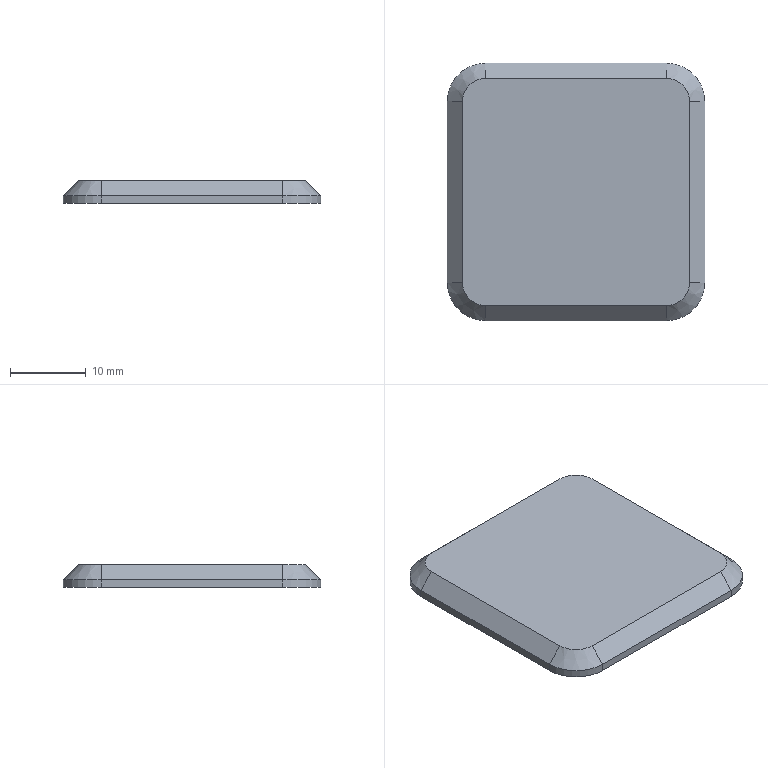Part | STEP file | IN-01-01-01-03 | 1 solid | 18 faces | box 34 x 34 x 3 mm | volume 3157 mm3 | plane 10 | cylinder 4 | cone 4 | commonest cylinder face diameters 10 x4
STEP:
#1=CARTESIAN_POINT('',(0.,0.,0.));
#2=DIRECTION('',(0.,0.,1.));
#3=DIRECTION('',(1.,0.,0.));
#4=AXIS2_PLACEMENT_3D('',#1,#2,#3);
#5=CARTESIAN_POINT('',(29.,-34.,0.));
#6=VERTEX_POINT('',#5);
#7=CARTESIAN_POINT('',(34.,-29.,0.));
#8=VERTEX_POINT('',#7);
#9=CARTESIAN_POINT('',(29.,-29.,0.));
#10=DIRECTION('',(0.,0.,1.));
#11=DIRECTION('',(1.,0.,0.));
#12=AXIS2_PLACEMENT_3D('',#9,#10,#11);
#13=CIRCLE('',#12,5.);
#14=CARTESIAN_POINT('',(17.,-17.,0.));
#15=DIRECTION('',(0.,0.,1.));
#16=DIRECTION('',(1.,0.,0.));
#17=AXIS2_PLACEMENT_3D('',#14,#15,#16);
#18=PLANE('',#17);
#19=CARTESIAN_POINT('',(12.,-12.));
#20=DIRECTION('',(1.,0.));
#21=AXIS2_PLACEMENT_2D('',#19,#20);
#22=CIRCLE('',#21,5.);
#23=(GEOMETRIC_REPRESENTATION_CONTEXT(2)PARAMETRIC_REPRESENTATION_CONTEXT()REPRESENTATION_CONTEXT('',''));
#24=DEFINITIONAL_REPRESENTATION('',(#22),#23);
#25=PCURVE('',#18,#24);
#26=CARTESIAN_POINT('',(29.,-29.,0.));
#27=DIRECTION('',(0.,0.,1.));
#28=DIRECTION('',(1.,0.,0.));
#29=AXIS2_PLACEMENT_3D('',#26,#27,#28);
#30=CYLINDRICAL_SURFACE('',#29,5.);
#31=CARTESIAN_POINT('',(0.,0.));
#32=DIRECTION('',(1.,0.));
#33=VECTOR('',#32,1.);
#34=LINE('',#31,#33);
#35=(GEOMETRIC_REPRESENTATION_CONTEXT(2)PARAMETRIC_REPRESENTATION_CONTEXT()REPRESENTATION_CONTEXT('',''));
#36=DEFINITIONAL_REPRESENTATION('',(#34),#35);
#37=PCURVE('',#30,#36);
#38=SURFACE_CURVE('',#13,(#25,#37),.PCURVE_S1.);
#39=EDGE_CURVE('',#6,#8,#38,.T.);
#40=ORIENTED_EDGE('',*,*,#39,.F.);
#41=CARTESIAN_POINT('',(5.,-34.,0.));
#42=VERTEX_POINT('',#41);
#43=CARTESIAN_POINT('',(17.,-34.,0.));
#44=DIRECTION('',(1.,0.,0.));
#45=VECTOR('',#44,1.);
#46=LINE('',#43,#45);
#47=CARTESIAN_POINT('',(0.,-17.));
#48=DIRECTION('',(1.,0.));
#49=VECTOR('',#48,1.);
#50=LINE('',#47,#49);
#51=(GEOMETRIC_REPRESENTATION_CONTEXT(2)PARAMETRIC_REPRESENTATION_CONTEXT()REPRESENTATION_CONTEXT('',''));
#52=DEFINITIONAL_REPRESENTATION('',(#50),#51);
#53=PCURVE('',#18,#52);
#54=CARTESIAN_POINT('',(5.,-34.,0.));
#55=DIRECTION('',(0.,-1.,0.));
#56=DIRECTION('',(1.,0.,0.));
#57=AXIS2_PLACEMENT_3D('',#54,#55,#56);
#58=PLANE('',#57);
#59=CARTESIAN_POINT('',(12.,0.));
#60=DIRECTION('',(1.,0.));
#61=VECTOR('',#60,1.);
#62=LINE('',#59,#61);
#63=(GEOMETRIC_REPRESENTATION_CONTEXT(2)PARAMETRIC_REPRESENTATION_CONTEXT()REPRESENTATION_CONTEXT('',''));
#64=DEFINITIONAL_REPRESENTATION('',(#62),#63);
#65=PCURVE('',#58,#64);
#66=SURFACE_CURVE('',#46,(#53,#65),.PCURVE_S1.);
#67=EDGE_CURVE('',#42,#6,#66,.T.);
#68=ORIENTED_EDGE('',*,*,#67,.F.);
#69=CARTESIAN_POINT('',(0.,-29.,0.));
#70=VERTEX_POINT('',#69);
#71=CARTESIAN_POINT('',(5.,-29.,0.));
#72=DIRECTION('',(0.,0.,1.));
#73=DIRECTION('',(1.,0.,0.));
#74=AXIS2_PLACEMENT_3D('',#71,#72,#73);
#75=CIRCLE('',#74,5.);
#76=CARTESIAN_POINT('',(-12.,-12.));
#77=DIRECTION('',(1.,0.));
#78=AXIS2_PLACEMENT_2D('',#76,#77);
#79=CIRCLE('',#78,5.);
#80=(GEOMETRIC_REPRESENTATION_CONTEXT(2)PARAMETRIC_REPRESENTATION_CONTEXT()REPRESENTATION_CONTEXT('',''));
#81=DEFINITIONAL_REPRESENTATION('',(#79),#80);
#82=PCURVE('',#18,#81);
#83=CARTESIAN_POINT('',(5.,-29.,0.));
#84=DIRECTION('',(0.,0.,1.));
#85=DIRECTION('',(1.,0.,0.));
#86=AXIS2_PLACEMENT_3D('',#83,#84,#85);
#87=CYLINDRICAL_SURFACE('',#86,5.);
#88=CARTESIAN_POINT('',(0.,0.));
#89=DIRECTION('',(1.,0.));
#90=VECTOR('',#89,1.);
#91=LINE('',#88,#90);
#92=(GEOMETRIC_REPRESENTATION_CONTEXT(2)PARAMETRIC_REPRESENTATION_CONTEXT()REPRESENTATION_CONTEXT('',''));
#93=DEFINITIONAL_REPRESENTATION('',(#91),#92);
#94=PCURVE('',#87,#93);
#95=SURFACE_CURVE('',#75,(#82,#94),.PCURVE_S1.);
#96=EDGE_CURVE('',#70,#42,#95,.T.);
#97=ORIENTED_EDGE('',*,*,#96,.F.);
#98=CARTESIAN_POINT('',(0.,-5.,0.));
#99=VERTEX_POINT('',#98);
#100=CARTESIAN_POINT('',(0.,-17.,0.));
#101=DIRECTION('',(0.,-1.,0.));
#102=VECTOR('',#101,1.);
#103=LINE('',#100,#102);
#104=CARTESIAN_POINT('',(-17.,0.));
#105=DIRECTION('',(0.,-1.));
#106=VECTOR('',#105,1.);
#107=LINE('',#104,#106);
#108=(GEOMETRIC_REPRESENTATION_CONTEXT(2)PARAMETRIC_REPRESENTATION_CONTEXT()REPRESENTATION_CONTEXT('',''));
#109=DEFINITIONAL_REPRESENTATION('',(#107),#108);
#110=PCURVE('',#18,#109);
#111=CARTESIAN_POINT('',(0.,-5.,0.));
#112=DIRECTION('',(-1.,0.,0.));
#113=DIRECTION('',(0.,-1.,0.));
#114=AXIS2_PLACEMENT_3D('',#111,#112,#113);
#115=PLANE('',#114);
#116=CARTESIAN_POINT('',(12.,0.));
#117=DIRECTION('',(1.,0.));
#118=VECTOR('',#117,1.);
#119=LINE('',#116,#118);
#120=(GEOMETRIC_REPRESENTATION_CONTEXT(2)PARAMETRIC_REPRESENTATION_CONTEXT()REPRESENTATION_CONTEXT('',''));
#121=DEFINITIONAL_REPRESENTATION('',(#119),#120);
#122=PCURVE('',#115,#121);
#123=SURFACE_CURVE('',#103,(#110,#122),.PCURVE_S1.);
#124=EDGE_CURVE('',#99,#70,#123,.T.);
#125=ORIENTED_EDGE('',*,*,#124,.F.);
#126=CARTESIAN_POINT('',(5.,0.,0.));
#127=VERTEX_POINT('',#126);
#128=CARTESIAN_POINT('',(5.,-5.,0.));
#129=DIRECTION('',(0.,0.,1.));
#130=DIRECTION('',(1.,0.,0.));
#131=AXIS2_PLACEMENT_3D('',#128,#129,#130);
#132=CIRCLE('',#131,5.);
#133=CARTESIAN_POINT('',(-12.,12.));
#134=DIRECTION('',(1.,0.));
#135=AXIS2_PLACEMENT_2D('',#133,#134);
#136=CIRCLE('',#135,5.);
#137=(GEOMETRIC_REPRESENTATION_CONTEXT(2)PARAMETRIC_REPRESENTATION_CONTEXT()REPRESENTATION_CONTEXT('',''));
#138=DEFINITIONAL_REPRESENTATION('',(#136),#137);
#139=PCURVE('',#18,#138);
#140=CARTESIAN_POINT('',(5.,-5.,0.));
#141=DIRECTION('',(0.,0.,1.));
#142=DIRECTION('',(1.,0.,0.));
#143=AXIS2_PLACEMENT_3D('',#140,#141,#142);
#144=CYLINDRICAL_SURFACE('',#143,5.);
#145=CARTESIAN_POINT('',(0.,0.));
#146=DIRECTION('',(1.,0.));
#147=VECTOR('',#146,1.);
#148=LINE('',#145,#147);
#149=(GEOMETRIC_REPRESENTATION_CONTEXT(2)PARAMETRIC_REPRESENTATION_CONTEXT()REPRESENTATION_CONTEXT('',''));
#150=DEFINITIONAL_REPRESENTATION('',(#148),#149);
#151=PCURVE('',#144,#150);
#152=SURFACE_CURVE('',#132,(#139,#151),.PCURVE_S1.);
#153=EDGE_CURVE('',#127,#99,#152,.T.);
#154=ORIENTED_EDGE('',*,*,#153,.F.);
#155=CARTESIAN_POINT('',(29.,0.,0.));
#156=VERTEX_POINT('',#155);
#157=CARTESIAN_POINT('',(17.,0.,0.));
#158=DIRECTION('',(-1.,0.,0.));
#159=VECTOR('',#158,1.);
#160=LINE('',#157,#159);
#161=CARTESIAN_POINT('',(0.,17.));
#162=DIRECTION('',(-1.,0.));
#163=VECTOR('',#162,1.);
#164=LINE('',#161,#163);
#165=(GEOMETRIC_REPRESENTATION_CONTEXT(2)PARAMETRIC_REPRESENTATION_CONTEXT()REPRESENTATION_CONTEXT('',''));
#166=DEFINITIONAL_REPRESENTATION('',(#164),#165);
#167=PCURVE('',#18,#166);
#168=CARTESIAN_POINT('',(29.,0.,0.));
#169=DIRECTION('',(0.,1.,0.));
#170=DIRECTION('',(-1.,0.,0.));
#171=AXIS2_PLACEMENT_3D('',#168,#169,#170);
#172=PLANE('',#171);
#173=CARTESIAN_POINT('',(12.,0.));
#174=DIRECTION('',(1.,0.));
#175=VECTOR('',#174,1.);
#176=LINE('',#173,#175);
#177=(GEOMETRIC_REPRESENTATION_CONTEXT(2)PARAMETRIC_REPRESENTATION_CONTEXT()REPRESENTATION_CONTEXT('',''));
#178=DEFINITIONAL_REPRESENTATION('',(#176),#177);
#179=PCURVE('',#172,#178);
#180=SURFACE_CURVE('',#160,(#167,#179),.PCURVE_S1.);
#181=EDGE_CURVE('',#156,#127,#180,.T.);
#182=ORIENTED_EDGE('',*,*,#181,.F.);
#183=CARTESIAN_POINT('',(34.,-5.,0.));
#184=VERTEX_POINT('',#183);
#185=CARTESIAN_POINT('',(29.,-5.,0.));
#186=DIRECTION('',(0.,0.,1.));
#187=DIRECTION('',(1.,0.,0.));
#188=AXIS2_PLACEMENT_3D('',#185,#186,#187);
#189=CIRCLE('',#188,5.);
#190=CARTESIAN_POINT('',(12.,12.));
#191=DIRECTION('',(1.,0.));
#192=AXIS2_PLACEMENT_2D('',#190,#191);
#193=CIRCLE('',#192,5.);
#194=(GEOMETRIC_REPRESENTATION_CONTEXT(2)PARAMETRIC_REPRESENTATION_CONTEXT()REPRESENTATION_CONTEXT('',''));
#195=DEFINITIONAL_REPRESENTATION('',(#193),#194);
#196=PCURVE('',#18,#195);
#197=CARTESIAN_POINT('',(29.,-5.,0.));
#198=DIRECTION('',(0.,0.,1.));
#199=DIRECTION('',(1.,0.,0.));
#200=AXIS2_PLACEMENT_3D('',#197,#198,#199);
#201=CYLINDRICAL_SURFACE('',#200,5.);
#202=CARTESIAN_POINT('',(0.,0.));
#203=DIRECTION('',(1.,0.));
#204=VECTOR('',#203,1.);
#205=LINE('',#202,#204);
#206=(GEOMETRIC_REPRESENTATION_CONTEXT(2)PARAMETRIC_REPRESENTATION_CONTEXT()REPRESENTATION_CONTEXT('',''));
#207=DEFINITIONAL_REPRESENTATION('',(#205),#206);
#208=PCURVE('',#201,#207);
#209=SURFACE_CURVE('',#189,(#196,#208),.PCURVE_S1.);
#210=EDGE_CURVE('',#184,#156,#209,.T.);
#211=ORIENTED_EDGE('',*,*,#210,.F.);
#212=CARTESIAN_POINT('',(34.,-17.,0.));
#213=DIRECTION('',(0.,1.,0.));
#214=VECTOR('',#213,1.);
#215=LINE('',#212,#214);
#216=CARTESIAN_POINT('',(17.,0.));
#217=DIRECTION('',(0.,1.));
#218=VECTOR('',#217,1.);
#219=LINE('',#216,#218);
#220=(GEOMETRIC_REPRESENTATION_CONTEXT(2)PARAMETRIC_REPRESENTATION_CONTEXT()REPRESENTATION_CONTEXT('',''));
#221=DEFINITIONAL_REPRESENTATION('',(#219),#220);
#222=PCURVE('',#18,#221);
#223=CARTESIAN_POINT('',(34.,-29.,0.));
#224=DIRECTION('',(1.,0.,0.));
#225=DIRECTION('',(0.,0.,-1.));
#226=AXIS2_PLACEMENT_3D('',#223,#224,#225);
#227=PLANE('',#226);
#228=CARTESIAN_POINT('',(0.,12.));
#229=DIRECTION('',(0.,1.));
#230=VECTOR('',#229,1.);
#231=LINE('',#228,#230);
#232=(GEOMETRIC_REPRESENTATION_CONTEXT(2)PARAMETRIC_REPRESENTATION_CONTEXT()REPRESENTATION_CONTEXT('',''));
#233=DEFINITIONAL_REPRESENTATION('',(#231),#232);
#234=PCURVE('',#227,#233);
#235=SURFACE_CURVE('',#215,(#222,#234),.PCURVE_S1.);
#236=EDGE_CURVE('',#8,#184,#235,.T.);
#237=ORIENTED_EDGE('',*,*,#236,.F.);
#238=EDGE_LOOP('',(#40,#68,#97,#125,#154,#182,#211,#237));
#239=FACE_BOUND('',#238,.T.);
#240=ADVANCED_FACE('',(#239),#18,.F.);
#241=ORIENTED_EDGE('',*,*,#236,.T.);
#242=CARTESIAN_POINT('',(34.,-5.,1.));
#243=VERTEX_POINT('',#242);
#244=CARTESIAN_POINT('',(34.,-5.,0.));
#245=DIRECTION('',(0.,0.,1.));
#246=VECTOR('',#245,1.);
#247=LINE('',#244,#246);
#248=CARTESIAN_POINT('',(0.,24.));
#249=DIRECTION('',(-1.,0.));
#250=VECTOR('',#249,1.);
#251=LINE('',#248,#250);
#252=(GEOMETRIC_REPRESENTATION_CONTEXT(2)PARAMETRIC_REPRESENTATION_CONTEXT()REPRESENTATION_CONTEXT('',''));
#253=DEFINITIONAL_REPRESENTATION('',(#251),#252);
#254=PCURVE('',#227,#253);
#255=CARTESIAN_POINT('',(0.,0.));
#256=DIRECTION('',(0.,1.));
#257=VECTOR('',#256,1.);
#258=LINE('',#255,#257);
#259=(GEOMETRIC_REPRESENTATION_CONTEXT(2)PARAMETRIC_REPRESENTATION_CONTEXT()REPRESENTATION_CONTEXT('',''));
#260=DEFINITIONAL_REPRESENTATION('',(#258),#259);
#261=PCURVE('',#201,#260);
#262=SURFACE_CURVE('',#247,(#254,#261),.PCURVE_S1.);
#263=EDGE_CURVE('',#184,#243,#262,.T.);
#264=ORIENTED_EDGE('',*,*,#263,.T.);
#265=CARTESIAN_POINT('',(34.,-29.,1.));
#266=VERTEX_POINT('',#265);
#267=CARTESIAN_POINT('',(34.,-29.,1.));
#268=DIRECTION('',(0.,-1.,0.));
#269=VECTOR('',#268,1.);
#270=LINE('',#267,#269);
#271=CARTESIAN_POINT('',(-1.,0.));
#272=DIRECTION('',(0.,-1.));
#273=VECTOR('',#272,1.);
#274=LINE('',#271,#273);
#275=(GEOMETRIC_REPRESENTATION_CONTEXT(2)PARAMETRIC_REPRESENTATION_CONTEXT()REPRESENTATION_CONTEXT('',''));
#276=DEFINITIONAL_REPRESENTATION('',(#274),#275);
#277=PCURVE('',#227,#276);
#278=CARTESIAN_POINT('',(33.,-23.,2.));
#279=DIRECTION('',(0.7071,0.,0.7071));
#280=DIRECTION('',(0.7071,0.,-0.7071));
#281=AXIS2_PLACEMENT_3D('',#278,#279,#280);
#282=PLANE('',#281);
#283=CARTESIAN_POINT('',(1.414,-6.));
#284=DIRECTION('',(0.,-1.));
#285=VECTOR('',#284,1.);
#286=LINE('',#283,#285);
#287=(GEOMETRIC_REPRESENTATION_CONTEXT(2)PARAMETRIC_REPRESENTATION_CONTEXT()REPRESENTATION_CONTEXT('',''));
#288=DEFINITIONAL_REPRESENTATION('',(#286),#287);
#289=PCURVE('',#282,#288);
#290=SURFACE_CURVE('',#270,(#277,#289),.PCURVE_S1.);
#291=EDGE_CURVE('',#243,#266,#290,.T.);
#292=ORIENTED_EDGE('',*,*,#291,.T.);
#293=CARTESIAN_POINT('',(34.,-29.,0.));
#294=DIRECTION('',(0.,0.,-1.));
#295=VECTOR('',#294,1.);
#296=LINE('',#293,#295);
#297=CARTESIAN_POINT('',(0.,0.));
#298=DIRECTION('',(1.,0.));
#299=VECTOR('',#298,1.);
#300=LINE('',#297,#299);
#301=(GEOMETRIC_REPRESENTATION_CONTEXT(2)PARAMETRIC_REPRESENTATION_CONTEXT()REPRESENTATION_CONTEXT('',''));
#302=DEFINITIONAL_REPRESENTATION('',(#300),#301);
#303=PCURVE('',#227,#302);
#304=CARTESIAN_POINT('',(6.283,0.));
#305=DIRECTION('',(0.,-1.));
#306=VECTOR('',#305,1.);
#307=LINE('',#304,#306);
#308=(GEOMETRIC_REPRESENTATION_CONTEXT(2)PARAMETRIC_REPRESENTATION_CONTEXT()REPRESENTATION_CONTEXT('',''));
#309=DEFINITIONAL_REPRESENTATION('',(#307),#308);
#310=PCURVE('',#30,#309);
#311=SURFACE_CURVE('',#296,(#303,#310),.PCURVE_S1.);
#312=EDGE_CURVE('',#266,#8,#311,.T.);
#313=ORIENTED_EDGE('',*,*,#312,.T.);
#314=EDGE_LOOP('',(#241,#264,#292,#313));
#315=FACE_BOUND('',#314,.T.);
#316=ADVANCED_FACE('',(#315),#227,.T.);
#317=ORIENTED_EDGE('',*,*,#39,.T.);
#318=ORIENTED_EDGE('',*,*,#312,.F.);
#319=CARTESIAN_POINT('',(29.,-34.,1.));
#320=VERTEX_POINT('',#319);
#321=CARTESIAN_POINT('',(29.,-29.,1.));
#322=DIRECTION('',(0.,0.,-1.));
#323=DIRECTION('',(1.,0.,0.));
#324=AXIS2_PLACEMENT_3D('',#321,#322,#323);
#325=CIRCLE('',#324,5.);
#326=CARTESIAN_POINT('',(6.283,1.));
#327=DIRECTION('',(-1.,0.));
#328=VECTOR('',#327,1.);
#329=LINE('',#326,#328);
#330=(GEOMETRIC_REPRESENTATION_CONTEXT(2)PARAMETRIC_REPRESENTATION_CONTEXT()REPRESENTATION_CONTEXT('',''));
#331=DEFINITIONAL_REPRESENTATION('',(#329),#330);
#332=PCURVE('',#30,#331);
#333=CARTESIAN_POINT('',(29.,-29.,1.));
#334=DIRECTION('',(0.,0.,-1.));
#335=DIRECTION('',(-1.,0.,0.));
#336=AXIS2_PLACEMENT_3D('',#333,#334,#335);
#337=CONICAL_SURFACE('',#336,5.,0.7854);
#338=CARTESIAN_POINT('',(3.142,0.));
#339=DIRECTION('',(1.,0.));
#340=VECTOR('',#339,1.);
#341=LINE('',#338,#340);
#342=(GEOMETRIC_REPRESENTATION_CONTEXT(2)PARAMETRIC_REPRESENTATION_CONTEXT()REPRESENTATION_CONTEXT('',''));
#343=DEFINITIONAL_REPRESENTATION('',(#341),#342);
#344=PCURVE('',#337,#343);
#345=SURFACE_CURVE('',#325,(#332,#344),.PCURVE_S1.);
#346=EDGE_CURVE('',#266,#320,#345,.T.);
#347=ORIENTED_EDGE('',*,*,#346,.T.);
#348=CARTESIAN_POINT('',(29.,-34.,0.));
#349=DIRECTION('',(0.,0.,-1.));
#350=VECTOR('',#349,1.);
#351=LINE('',#348,#350);
#352=CARTESIAN_POINT('',(4.712,0.));
#353=DIRECTION('',(0.,-1.));
#354=VECTOR('',#353,1.);
#355=LINE('',#352,#354);
#356=(GEOMETRIC_REPRESENTATION_CONTEXT(2)PARAMETRIC_REPRESENTATION_CONTEXT()REPRESENTATION_CONTEXT('',''));
#357=DEFINITIONAL_REPRESENTATION('',(#355),#356);
#358=PCURVE('',#30,#357);
#359=CARTESIAN_POINT('',(24.,0.));
#360=DIRECTION('',(0.,-1.));
#361=VECTOR('',#360,1.);
#362=LINE('',#359,#361);
#363=(GEOMETRIC_REPRESENTATION_CONTEXT(2)PARAMETRIC_REPRESENTATION_CONTEXT()REPRESENTATION_CONTEXT('',''));
#364=DEFINITIONAL_REPRESENTATION('',(#362),#363);
#365=PCURVE('',#58,#364);
#366=SURFACE_CURVE('',#351,(#358,#365),.PCURVE_S1.);
#367=EDGE_CURVE('',#320,#6,#366,.T.);
#368=ORIENTED_EDGE('',*,*,#367,.T.);
#369=EDGE_LOOP('',(#317,#318,#347,#368));
#370=FACE_BOUND('',#369,.T.);
#371=ADVANCED_FACE('',(#370),#30,.T.);
#372=ORIENTED_EDGE('',*,*,#67,.T.);
#373=ORIENTED_EDGE('',*,*,#367,.F.);
#374=CARTESIAN_POINT('',(5.,-34.,1.));
#375=VERTEX_POINT('',#374);
#376=CARTESIAN_POINT('',(5.,-34.,1.));
#377=DIRECTION('',(-1.,0.,0.));
#378=VECTOR('',#377,1.);
#379=LINE('',#376,#378);
#380=CARTESIAN_POINT('',(0.,1.));
#381=DIRECTION('',(-1.,0.));
#382=VECTOR('',#381,1.);
#383=LINE('',#380,#382);
#384=(GEOMETRIC_REPRESENTATION_CONTEXT(2)PARAMETRIC_REPRESENTATION_CONTEXT()REPRESENTATION_CONTEXT('',''));
#385=DEFINITIONAL_REPRESENTATION('',(#383),#384);
#386=PCURVE('',#58,#385);
#387=CARTESIAN_POINT('',(11.,-33.,2.));
#388=DIRECTION('',(0.,-0.7071,0.7071));
#389=DIRECTION('',(0.,-0.7071,-0.7071));
#390=AXIS2_PLACEMENT_3D('',#387,#388,#389);
#391=PLANE('',#390);
#392=CARTESIAN_POINT('',(1.414,-6.));
#393=DIRECTION('',(0.,-1.));
#394=VECTOR('',#393,1.);
#395=LINE('',#392,#394);
#396=(GEOMETRIC_REPRESENTATION_CONTEXT(2)PARAMETRIC_REPRESENTATION_CONTEXT()REPRESENTATION_CONTEXT('',''));
#397=DEFINITIONAL_REPRESENTATION('',(#395),#396);
#398=PCURVE('',#391,#397);
#399=SURFACE_CURVE('',#379,(#386,#398),.PCURVE_S1.);
#400=EDGE_CURVE('',#320,#375,#399,.T.);
#401=ORIENTED_EDGE('',*,*,#400,.T.);
#402=CARTESIAN_POINT('',(5.,-34.,0.));
#403=DIRECTION('',(0.,0.,-1.));
#404=VECTOR('',#403,1.);
#405=LINE('',#402,#404);
#406=CARTESIAN_POINT('',(0.,0.));
#407=DIRECTION('',(0.,-1.));
#408=VECTOR('',#407,1.);
#409=LINE('',#406,#408);
#410=(GEOMETRIC_REPRESENTATION_CONTEXT(2)PARAMETRIC_REPRESENTATION_CONTEXT()REPRESENTATION_CONTEXT('',''));
#411=DEFINITIONAL_REPRESENTATION('',(#409),#410);
#412=PCURVE('',#58,#411);
#413=CARTESIAN_POINT('',(4.712,0.));
#414=DIRECTION('',(0.,-1.));
#415=VECTOR('',#414,1.);
#416=LINE('',#413,#415);
#417=(GEOMETRIC_REPRESENTATION_CONTEXT(2)PARAMETRIC_REPRESENTATION_CONTEXT()REPRESENTATION_CONTEXT('',''));
#418=DEFINITIONAL_REPRESENTATION('',(#416),#417);
#419=PCURVE('',#87,#418);
#420=SURFACE_CURVE('',#405,(#412,#419),.PCURVE_S1.);
#421=EDGE_CURVE('',#375,#42,#420,.T.);
#422=ORIENTED_EDGE('',*,*,#421,.T.);
#423=EDGE_LOOP('',(#372,#373,#401,#422));
#424=FACE_BOUND('',#423,.T.);
#425=ADVANCED_FACE('',(#424),#58,.T.);
#426=ORIENTED_EDGE('',*,*,#96,.T.);
#427=ORIENTED_EDGE('',*,*,#421,.F.);
#428=CARTESIAN_POINT('',(0.,-29.,1.));
#429=VERTEX_POINT('',#428);
#430=CARTESIAN_POINT('',(5.,-29.,1.));
#431=DIRECTION('',(0.,0.,-1.));
#432=DIRECTION('',(1.,0.,0.));
#433=AXIS2_PLACEMENT_3D('',#430,#431,#432);
#434=CIRCLE('',#433,5.);
#435=CARTESIAN_POINT('',(6.283,1.));
#436=DIRECTION('',(-1.,0.));
#437=VECTOR('',#436,1.);
#438=LINE('',#435,#437);
#439=(GEOMETRIC_REPRESENTATION_CONTEXT(2)PARAMETRIC_REPRESENTATION_CONTEXT()REPRESENTATION_CONTEXT('',''));
#440=DEFINITIONAL_REPRESENTATION('',(#438),#439);
#441=PCURVE('',#87,#440);
#442=CARTESIAN_POINT('',(5.,-29.,1.));
#443=DIRECTION('',(0.,0.,-1.));
#444=DIRECTION('',(-1.,0.,0.));
#445=AXIS2_PLACEMENT_3D('',#442,#443,#444);
#446=CONICAL_SURFACE('',#445,5.,0.7854);
#447=CARTESIAN_POINT('',(3.142,0.));
#448=DIRECTION('',(1.,0.));
#449=VECTOR('',#448,1.);
#450=LINE('',#447,#449);
#451=(GEOMETRIC_REPRESENTATION_CONTEXT(2)PARAMETRIC_REPRESENTATION_CONTEXT()REPRESENTATION_CONTEXT('',''));
#452=DEFINITIONAL_REPRESENTATION('',(#450),#451);
#453=PCURVE('',#446,#452);
#454=SURFACE_CURVE('',#434,(#441,#453),.PCURVE_S1.);
#455=EDGE_CURVE('',#375,#429,#454,.T.);
#456=ORIENTED_EDGE('',*,*,#455,.T.);
#457=CARTESIAN_POINT('',(0.,-29.,0.));
#458=DIRECTION('',(0.,0.,-1.));
#459=VECTOR('',#458,1.);
#460=LINE('',#457,#459);
#461=CARTESIAN_POINT('',(3.142,0.));
#462=DIRECTION('',(0.,-1.));
#463=VECTOR('',#462,1.);
#464=LINE('',#461,#463);
#465=(GEOMETRIC_REPRESENTATION_CONTEXT(2)PARAMETRIC_REPRESENTATION_CONTEXT()REPRESENTATION_CONTEXT('',''));
#466=DEFINITIONAL_REPRESENTATION('',(#464),#465);
#467=PCURVE('',#87,#466);
#468=CARTESIAN_POINT('',(24.,0.));
#469=DIRECTION('',(0.,-1.));
#470=VECTOR('',#469,1.);
#471=LINE('',#468,#470);
#472=(GEOMETRIC_REPRESENTATION_CONTEXT(2)PARAMETRIC_REPRESENTATION_CONTEXT()REPRESENTATION_CONTEXT('',''));
#473=DEFINITIONAL_REPRESENTATION('',(#471),#472);
#474=PCURVE('',#115,#473);
#475=SURFACE_CURVE('',#460,(#467,#474),.PCURVE_S1.);
#476=EDGE_CURVE('',#429,#70,#475,.T.);
#477=ORIENTED_EDGE('',*,*,#476,.T.);
#478=EDGE_LOOP('',(#426,#427,#456,#477));
#479=FACE_BOUND('',#478,.T.);
#480=ADVANCED_FACE('',(#479),#87,.T.);
#481=ORIENTED_EDGE('',*,*,#124,.T.);
#482=ORIENTED_EDGE('',*,*,#476,.F.);
#483=CARTESIAN_POINT('',(0.,-5.,1.));
#484=VERTEX_POINT('',#483);
#485=CARTESIAN_POINT('',(0.,-5.,1.));
#486=DIRECTION('',(0.,1.,0.));
#487=VECTOR('',#486,1.);
#488=LINE('',#485,#487);
#489=CARTESIAN_POINT('',(0.,1.));
#490=DIRECTION('',(-1.,0.));
#491=VECTOR('',#490,1.);
#492=LINE('',#489,#491);
#493=(GEOMETRIC_REPRESENTATION_CONTEXT(2)PARAMETRIC_REPRESENTATION_CONTEXT()REPRESENTATION_CONTEXT('',''));
#494=DEFINITIONAL_REPRESENTATION('',(#492),#493);
#495=PCURVE('',#115,#494);
#496=CARTESIAN_POINT('',(1.,-11.,2.));
#497=DIRECTION('',(-0.7071,0.,0.7071));
#498=DIRECTION('',(0.7071,0.,0.7071));
#499=AXIS2_PLACEMENT_3D('',#496,#497,#498);
#500=PLANE('',#499);
#501=CARTESIAN_POINT('',(-1.414,6.));
#502=DIRECTION('',(0.,1.));
#503=VECTOR('',#502,1.);
#504=LINE('',#501,#503);
#505=(GEOMETRIC_REPRESENTATION_CONTEXT(2)PARAMETRIC_REPRESENTATION_CONTEXT()REPRESENTATION_CONTEXT('',''));
#506=DEFINITIONAL_REPRESENTATION('',(#504),#505);
#507=PCURVE('',#500,#506);
#508=SURFACE_CURVE('',#488,(#495,#507),.PCURVE_S1.);
#509=EDGE_CURVE('',#429,#484,#508,.T.);
#510=ORIENTED_EDGE('',*,*,#509,.T.);
#511=CARTESIAN_POINT('',(0.,-5.,0.));
#512=DIRECTION('',(0.,0.,-1.));
#513=VECTOR('',#512,1.);
#514=LINE('',#511,#513);
#515=CARTESIAN_POINT('',(0.,0.));
#516=DIRECTION('',(0.,-1.));
#517=VECTOR('',#516,1.);
#518=LINE('',#515,#517);
#519=(GEOMETRIC_REPRESENTATION_CONTEXT(2)PARAMETRIC_REPRESENTATION_CONTEXT()REPRESENTATION_CONTEXT('',''));
#520=DEFINITIONAL_REPRESENTATION('',(#518),#519);
#521=PCURVE('',#115,#520);
#522=CARTESIAN_POINT('',(3.142,0.));
#523=DIRECTION('',(0.,-1.));
#524=VECTOR('',#523,1.);
#525=LINE('',#522,#524);
#526=(GEOMETRIC_REPRESENTATION_CONTEXT(2)PARAMETRIC_REPRESENTATION_CONTEXT()REPRESENTATION_CONTEXT('',''));
#527=DEFINITIONAL_REPRESENTATION('',(#525),#526);
#528=PCURVE('',#144,#527);
#529=SURFACE_CURVE('',#514,(#521,#528),.PCURVE_S1.);
#530=EDGE_CURVE('',#484,#99,#529,.T.);
#531=ORIENTED_EDGE('',*,*,#530,.T.);
#532=EDGE_LOOP('',(#481,#482,#510,#531));
#533=FACE_BOUND('',#532,.T.);
#534=ADVANCED_FACE('',(#533),#115,.T.);
#535=ORIENTED_EDGE('',*,*,#153,.T.);
#536=ORIENTED_EDGE('',*,*,#530,.F.);
#537=CARTESIAN_POINT('',(5.,0.,1.));
#538=VERTEX_POINT('',#537);
#539=CARTESIAN_POINT('',(5.,-5.,1.));
#540=DIRECTION('',(0.,0.,-1.));
#541=DIRECTION('',(1.,0.,0.));
#542=AXIS2_PLACEMENT_3D('',#539,#540,#541);
#543=CIRCLE('',#542,5.);
#544=CARTESIAN_POINT('',(6.283,1.));
#545=DIRECTION('',(-1.,0.));
#546=VECTOR('',#545,1.);
#547=LINE('',#544,#546);
#548=(GEOMETRIC_REPRESENTATION_CONTEXT(2)PARAMETRIC_REPRESENTATION_CONTEXT()REPRESENTATION_CONTEXT('',''));
#549=DEFINITIONAL_REPRESENTATION('',(#547),#548);
#550=PCURVE('',#144,#549);
#551=CARTESIAN_POINT('',(5.,-5.,1.));
#552=DIRECTION('',(0.,0.,-1.));
#553=DIRECTION('',(-1.,0.,0.));
#554=AXIS2_PLACEMENT_3D('',#551,#552,#553);
#555=CONICAL_SURFACE('',#554,5.,0.7854);
#556=CARTESIAN_POINT('',(-3.142,0.));
#557=DIRECTION('',(1.,0.));
#558=VECTOR('',#557,1.);
#559=LINE('',#556,#558);
#560=(GEOMETRIC_REPRESENTATION_CONTEXT(2)PARAMETRIC_REPRESENTATION_CONTEXT()REPRESENTATION_CONTEXT('',''));
#561=DEFINITIONAL_REPRESENTATION('',(#559),#560);
#562=PCURVE('',#555,#561);
#563=SURFACE_CURVE('',#543,(#550,#562),.PCURVE_S1.);
#564=EDGE_CURVE('',#484,#538,#563,.T.);
#565=ORIENTED_EDGE('',*,*,#564,.T.);
#566=CARTESIAN_POINT('',(5.,0.,0.));
#567=DIRECTION('',(0.,0.,-1.));
#568=VECTOR('',#567,1.);
#569=LINE('',#566,#568);
#570=CARTESIAN_POINT('',(1.571,0.));
#571=DIRECTION('',(0.,-1.));
#572=VECTOR('',#571,1.);
#573=LINE('',#570,#572);
#574=(GEOMETRIC_REPRESENTATION_CONTEXT(2)PARAMETRIC_REPRESENTATION_CONTEXT()REPRESENTATION_CONTEXT('',''));
#575=DEFINITIONAL_REPRESENTATION('',(#573),#574);
#576=PCURVE('',#144,#575);
#577=CARTESIAN_POINT('',(24.,0.));
#578=DIRECTION('',(0.,-1.));
#579=VECTOR('',#578,1.);
#580=LINE('',#577,#579);
#581=(GEOMETRIC_REPRESENTATION_CONTEXT(2)PARAMETRIC_REPRESENTATION_CONTEXT()REPRESENTATION_CONTEXT('',''));
#582=DEFINITIONAL_REPRESENTATION('',(#580),#581);
#583=PCURVE('',#172,#582);
#584=SURFACE_CURVE('',#569,(#576,#583),.PCURVE_S1.);
#585=EDGE_CURVE('',#538,#127,#584,.T.);
#586=ORIENTED_EDGE('',*,*,#585,.T.);
#587=EDGE_LOOP('',(#535,#536,#565,#586));
#588=FACE_BOUND('',#587,.T.);
#589=ADVANCED_FACE('',(#588),#144,.T.);
#590=ORIENTED_EDGE('',*,*,#181,.T.);
#591=ORIENTED_EDGE('',*,*,#585,.F.);
#592=CARTESIAN_POINT('',(29.,0.,1.));
#593=VERTEX_POINT('',#592);
#594=CARTESIAN_POINT('',(29.,0.,1.));
#595=DIRECTION('',(1.,0.,0.));
#596=VECTOR('',#595,1.);
#597=LINE('',#594,#596);
#598=CARTESIAN_POINT('',(0.,1.));
#599=DIRECTION('',(-1.,0.));
#600=VECTOR('',#599,1.);
#601=LINE('',#598,#600);
#602=(GEOMETRIC_REPRESENTATION_CONTEXT(2)PARAMETRIC_REPRESENTATION_CONTEXT()REPRESENTATION_CONTEXT('',''));
#603=DEFINITIONAL_REPRESENTATION('',(#601),#602);
#604=PCURVE('',#172,#603);
#605=CARTESIAN_POINT('',(23.,-1.,2.));
#606=DIRECTION('',(0.,0.7071,0.7071));
#607=DIRECTION('',(0.,-0.7071,0.7071));
#608=AXIS2_PLACEMENT_3D('',#605,#606,#607);
#609=PLANE('',#608);
#610=CARTESIAN_POINT('',(-1.414,6.));
#611=DIRECTION('',(0.,1.));
#612=VECTOR('',#611,1.);
#613=LINE('',#610,#612);
#614=(GEOMETRIC_REPRESENTATION_CONTEXT(2)PARAMETRIC_REPRESENTATION_CONTEXT()REPRESENTATION_CONTEXT('',''));
#615=DEFINITIONAL_REPRESENTATION('',(#613),#614);
#616=PCURVE('',#609,#615);
#617=SURFACE_CURVE('',#597,(#604,#616),.PCURVE_S1.);
#618=EDGE_CURVE('',#538,#593,#617,.T.);
#619=ORIENTED_EDGE('',*,*,#618,.T.);
#620=CARTESIAN_POINT('',(29.,0.,0.));
#621=DIRECTION('',(0.,0.,-1.));
#622=VECTOR('',#621,1.);
#623=LINE('',#620,#622);
#624=CARTESIAN_POINT('',(0.,0.));
#625=DIRECTION('',(0.,-1.));
#626=VECTOR('',#625,1.);
#627=LINE('',#624,#626);
#628=(GEOMETRIC_REPRESENTATION_CONTEXT(2)PARAMETRIC_REPRESENTATION_CONTEXT()REPRESENTATION_CONTEXT('',''));
#629=DEFINITIONAL_REPRESENTATION('',(#627),#628);
#630=PCURVE('',#172,#629);
#631=CARTESIAN_POINT('',(1.571,0.));
#632=DIRECTION('',(0.,-1.));
#633=VECTOR('',#632,1.);
#634=LINE('',#631,#633);
#635=(GEOMETRIC_REPRESENTATION_CONTEXT(2)PARAMETRIC_REPRESENTATION_CONTEXT()REPRESENTATION_CONTEXT('',''));
#636=DEFINITIONAL_REPRESENTATION('',(#634),#635);
#637=PCURVE('',#201,#636);
#638=SURFACE_CURVE('',#623,(#630,#637),.PCURVE_S1.);
#639=EDGE_CURVE('',#593,#156,#638,.T.);
#640=ORIENTED_EDGE('',*,*,#639,.T.);
#641=EDGE_LOOP('',(#590,#591,#619,#640));
#642=FACE_BOUND('',#641,.T.);
#643=ADVANCED_FACE('',(#642),#172,.T.);
#644=ORIENTED_EDGE('',*,*,#210,.T.);
#645=ORIENTED_EDGE('',*,*,#639,.F.);
#646=CARTESIAN_POINT('',(29.,-5.,1.));
#647=DIRECTION('',(0.,0.,-1.));
#648=DIRECTION('',(1.,0.,0.));
#649=AXIS2_PLACEMENT_3D('',#646,#647,#648);
#650=CIRCLE('',#649,5.);
#651=CARTESIAN_POINT('',(6.283,1.));
#652=DIRECTION('',(-1.,0.));
#653=VECTOR('',#652,1.);
#654=LINE('',#651,#653);
#655=(GEOMETRIC_REPRESENTATION_CONTEXT(2)PARAMETRIC_REPRESENTATION_CONTEXT()REPRESENTATION_CONTEXT('',''));
#656=DEFINITIONAL_REPRESENTATION('',(#654),#655);
#657=PCURVE('',#201,#656);
#658=CARTESIAN_POINT('',(29.,-5.,1.));
#659=DIRECTION('',(0.,0.,-1.));
#660=DIRECTION('',(-1.,0.,0.));
#661=AXIS2_PLACEMENT_3D('',#658,#659,#660);
#662=CONICAL_SURFACE('',#661,5.,0.7854);
#663=CARTESIAN_POINT('',(-3.142,0.));
#664=DIRECTION('',(1.,0.));
#665=VECTOR('',#664,1.);
#666=LINE('',#663,#665);
#667=(GEOMETRIC_REPRESENTATION_CONTEXT(2)PARAMETRIC_REPRESENTATION_CONTEXT()REPRESENTATION_CONTEXT('',''));
#668=DEFINITIONAL_REPRESENTATION('',(#666),#667);
#669=PCURVE('',#662,#668);
#670=SURFACE_CURVE('',#650,(#657,#669),.PCURVE_S1.);
#671=EDGE_CURVE('',#593,#243,#670,.T.);
#672=ORIENTED_EDGE('',*,*,#671,.T.);
#673=ORIENTED_EDGE('',*,*,#263,.F.);
#674=EDGE_LOOP('',(#644,#645,#672,#673));
#675=FACE_BOUND('',#674,.T.);
#676=ADVANCED_FACE('',(#675),#201,.T.);
#677=CARTESIAN_POINT('',(32.,-29.,3.));
#678=VERTEX_POINT('',#677);
#679=CARTESIAN_POINT('',(33.,-29.,2.));
#680=DIRECTION('',(0.7071,0.,-0.7071));
#681=VECTOR('',#680,1.);
#682=LINE('',#679,#681);
#683=CARTESIAN_POINT('',(0.,-6.));
#684=DIRECTION('',(1.,0.));
#685=VECTOR('',#684,1.);
#686=LINE('',#683,#685);
#687=(GEOMETRIC_REPRESENTATION_CONTEXT(2)PARAMETRIC_REPRESENTATION_CONTEXT()REPRESENTATION_CONTEXT('',''));
#688=DEFINITIONAL_REPRESENTATION('',(#686),#687);
#689=PCURVE('',#282,#688);
#690=CARTESIAN_POINT('',(3.142,-1.));
#691=DIRECTION('',(0.,1.));
#692=VECTOR('',#691,1.);
#693=LINE('',#690,#692);
#694=(GEOMETRIC_REPRESENTATION_CONTEXT(2)PARAMETRIC_REPRESENTATION_CONTEXT()REPRESENTATION_CONTEXT('',''));
#695=DEFINITIONAL_REPRESENTATION('',(#693),#694);
#696=PCURVE('',#337,#695);
#697=SURFACE_CURVE('',#682,(#689,#696),.PCURVE_S1.);
#698=EDGE_CURVE('',#678,#266,#697,.T.);
#699=ORIENTED_EDGE('',*,*,#698,.T.);
#700=ORIENTED_EDGE('',*,*,#291,.F.);
#701=CARTESIAN_POINT('',(32.,-5.,3.));
#702=VERTEX_POINT('',#701);
#703=CARTESIAN_POINT('',(33.,-5.,2.));
#704=DIRECTION('',(-0.7071,0.,0.7071));
#705=VECTOR('',#704,1.);
#706=LINE('',#703,#705);
#707=CARTESIAN_POINT('',(0.,18.));
#708=DIRECTION('',(-1.,0.));
#709=VECTOR('',#708,1.);
#710=LINE('',#707,#709);
#711=(GEOMETRIC_REPRESENTATION_CONTEXT(2)PARAMETRIC_REPRESENTATION_CONTEXT()REPRESENTATION_CONTEXT('',''));
#712=DEFINITIONAL_REPRESENTATION('',(#710),#711);
#713=PCURVE('',#282,#712);
#714=CARTESIAN_POINT('',(3.142,-1.));
#715=DIRECTION('',(0.,-1.));
#716=VECTOR('',#715,1.);
#717=LINE('',#714,#716);
#718=(GEOMETRIC_REPRESENTATION_CONTEXT(2)PARAMETRIC_REPRESENTATION_CONTEXT()REPRESENTATION_CONTEXT('',''));
#719=DEFINITIONAL_REPRESENTATION('',(#717),#718);
#720=PCURVE('',#662,#719);
#721=SURFACE_CURVE('',#706,(#713,#720),.PCURVE_S1.);
#722=EDGE_CURVE('',#243,#702,#721,.T.);
#723=ORIENTED_EDGE('',*,*,#722,.T.);
#724=CARTESIAN_POINT('',(32.,-23.,3.));
#725=DIRECTION('',(0.,-1.,0.));
#726=VECTOR('',#725,1.);
#727=LINE('',#724,#726);
#728=CARTESIAN_POINT('',(-1.414,0.));
#729=DIRECTION('',(0.,-1.));
#730=VECTOR('',#729,1.);
#731=LINE('',#728,#730);
#732=(GEOMETRIC_REPRESENTATION_CONTEXT(2)PARAMETRIC_REPRESENTATION_CONTEXT()REPRESENTATION_CONTEXT('',''));
#733=DEFINITIONAL_REPRESENTATION('',(#731),#732);
#734=PCURVE('',#282,#733);
#735=CARTESIAN_POINT('',(17.,-17.,3.));
#736=DIRECTION('',(0.,0.,1.));
#737=DIRECTION('',(1.,0.,0.));
#738=AXIS2_PLACEMENT_3D('',#735,#736,#737);
#739=PLANE('',#738);
#740=CARTESIAN_POINT('',(15.,-6.));
#741=DIRECTION('',(0.,-1.));
#742=VECTOR('',#741,1.);
#743=LINE('',#740,#742);
#744=(GEOMETRIC_REPRESENTATION_CONTEXT(2)PARAMETRIC_REPRESENTATION_CONTEXT()REPRESENTATION_CONTEXT('',''));
#745=DEFINITIONAL_REPRESENTATION('',(#743),#744);
#746=PCURVE('',#739,#745);
#747=SURFACE_CURVE('',#727,(#734,#746),.PCURVE_S1.);
#748=EDGE_CURVE('',#702,#678,#747,.T.);
#749=ORIENTED_EDGE('',*,*,#748,.T.);
#750=EDGE_LOOP('',(#699,#700,#723,#749));
#751=FACE_BOUND('',#750,.T.);
#752=ADVANCED_FACE('',(#751),#282,.T.);
#753=CARTESIAN_POINT('',(29.,-32.,3.));
#754=VERTEX_POINT('',#753);
#755=CARTESIAN_POINT('',(29.,-499000.,-498965.));
#756=DIRECTION('',(0.,-0.7071,-0.7071));
#757=VECTOR('',#756,1.);
#758=LINE('',#755,#757);
#759=CARTESIAN_POINT('',(4.712,498966.));
#760=DIRECTION('',(0.,1.));
#761=VECTOR('',#760,1.);
#762=LINE('',#759,#761);
#763=(GEOMETRIC_REPRESENTATION_CONTEXT(2)PARAMETRIC_REPRESENTATION_CONTEXT()REPRESENTATION_CONTEXT('',''));
#764=DEFINITIONAL_REPRESENTATION('',(#762),#763);
#765=PCURVE('',#337,#764);
#766=CARTESIAN_POINT('',(705645.899,18.));
#767=DIRECTION('',(1.,0.));
#768=VECTOR('',#767,1.);
#769=LINE('',#766,#768);
#770=(GEOMETRIC_REPRESENTATION_CONTEXT(2)PARAMETRIC_REPRESENTATION_CONTEXT()REPRESENTATION_CONTEXT('',''));
#771=DEFINITIONAL_REPRESENTATION('',(#769),#770);
#772=PCURVE('',#391,#771);
#773=SURFACE_CURVE('',#758,(#765,#772),.PCURVE_S1.);
#774=EDGE_CURVE('',#754,#320,#773,.T.);
#775=ORIENTED_EDGE('',*,*,#774,.T.);
#776=ORIENTED_EDGE('',*,*,#346,.F.);
#777=ORIENTED_EDGE('',*,*,#698,.F.);
#778=CARTESIAN_POINT('',(29.,-29.,3.));
#779=DIRECTION('',(0.,0.,-1.));
#780=DIRECTION('',(-1.,0.,0.));
#781=AXIS2_PLACEMENT_3D('',#778,#779,#780);
#782=CIRCLE('',#781,3.);
#783=CARTESIAN_POINT('',(0.,-2.));
#784=DIRECTION('',(1.,0.));
#785=VECTOR('',#784,1.);
#786=LINE('',#783,#785);
#787=(GEOMETRIC_REPRESENTATION_CONTEXT(2)PARAMETRIC_REPRESENTATION_CONTEXT()REPRESENTATION_CONTEXT('',''));
#788=DEFINITIONAL_REPRESENTATION('',(#786),#787);
#789=PCURVE('',#337,#788);
#790=CARTESIAN_POINT('',(9.,-12.));
#791=CARTESIAN_POINT('',(9.,-6.804));
#792=CARTESIAN_POINT('',(13.5,-9.402));
#793=CARTESIAN_POINT('',(18.,-12.));
#794=CARTESIAN_POINT('',(13.5,-14.598));
#795=CARTESIAN_POINT('',(9.,-17.196));
#796=CARTESIAN_POINT('',(9.,-12.));
#797=(BOUNDED_CURVE()B_SPLINE_CURVE(2,(#790,#791,#792,#793,#794,#795,#796),.UNSPECIFIED.,.T.,.F.)B_SPLINE_CURVE_WITH_KNOTS((1,2,2,2,2,1),(-2.094,0.,2.094,4.189,6.283,8.378),.UNSPECIFIED.)CURVE()GEOMETRIC_REPRESENTATION_ITEM()RATIONAL_B_SPLINE_CURVE((1.,0.5,1.,0.5,1.,0.5,1.))REPRESENTATION_ITEM(''));
#798=(GEOMETRIC_REPRESENTATION_CONTEXT(2)PARAMETRIC_REPRESENTATION_CONTEXT()REPRESENTATION_CONTEXT('',''));
#799=DEFINITIONAL_REPRESENTATION('',(#797),#798);
#800=PCURVE('',#739,#799);
#801=SURFACE_CURVE('',#782,(#789,#800),.PCURVE_S1.);
#802=EDGE_CURVE('',#678,#754,#801,.T.);
#803=ORIENTED_EDGE('',*,*,#802,.T.);
#804=EDGE_LOOP('',(#775,#776,#777,#803));
#805=FACE_BOUND('',#804,.T.);
#806=ADVANCED_FACE('',(#805),#337,.T.);
#807=CARTESIAN_POINT('',(5.,-32.,3.));
#808=VERTEX_POINT('',#807);
#809=CARTESIAN_POINT('',(5.,-33.,2.));
#810=DIRECTION('',(0.,-0.7071,-0.7071));
#811=VECTOR('',#810,1.);
#812=LINE('',#809,#811);
#813=CARTESIAN_POINT('',(0.,-6.));
#814=DIRECTION('',(1.,0.));
#815=VECTOR('',#814,1.);
#816=LINE('',#813,#815);
#817=(GEOMETRIC_REPRESENTATION_CONTEXT(2)PARAMETRIC_REPRESENTATION_CONTEXT()REPRESENTATION_CONTEXT('',''));
#818=DEFINITIONAL_REPRESENTATION('',(#816),#817);
#819=PCURVE('',#391,#818);
#820=CARTESIAN_POINT('',(4.712,-1.));
#821=DIRECTION('',(0.,1.));
#822=VECTOR('',#821,1.);
#823=LINE('',#820,#822);
#824=(GEOMETRIC_REPRESENTATION_CONTEXT(2)PARAMETRIC_REPRESENTATION_CONTEXT()REPRESENTATION_CONTEXT('',''));
#825=DEFINITIONAL_REPRESENTATION('',(#823),#824);
#826=PCURVE('',#446,#825);
#827=SURFACE_CURVE('',#812,(#819,#826),.PCURVE_S1.);
#828=EDGE_CURVE('',#808,#375,#827,.T.);
#829=ORIENTED_EDGE('',*,*,#828,.T.);
#830=ORIENTED_EDGE('',*,*,#400,.F.);
#831=ORIENTED_EDGE('',*,*,#774,.F.);
#832=CARTESIAN_POINT('',(11.,-32.,3.));
#833=DIRECTION('',(-1.,0.,0.));
#834=VECTOR('',#833,1.);
#835=LINE('',#832,#834);
#836=CARTESIAN_POINT('',(-1.414,0.));
#837=DIRECTION('',(0.,-1.));
#838=VECTOR('',#837,1.);
#839=LINE('',#836,#838);
#840=(GEOMETRIC_REPRESENTATION_CONTEXT(2)PARAMETRIC_REPRESENTATION_CONTEXT()REPRESENTATION_CONTEXT('',''));
#841=DEFINITIONAL_REPRESENTATION('',(#839),#840);
#842=PCURVE('',#391,#841);
#843=CARTESIAN_POINT('',(-6.,-15.));
#844=DIRECTION('',(-1.,0.));
#845=VECTOR('',#844,1.);
#846=LINE('',#843,#845);
#847=(GEOMETRIC_REPRESENTATION_CONTEXT(2)PARAMETRIC_REPRESENTATION_CONTEXT()REPRESENTATION_CONTEXT('',''));
#848=DEFINITIONAL_REPRESENTATION('',(#846),#847);
#849=PCURVE('',#739,#848);
#850=SURFACE_CURVE('',#835,(#842,#849),.PCURVE_S1.);
#851=EDGE_CURVE('',#754,#808,#850,.T.);
#852=ORIENTED_EDGE('',*,*,#851,.T.);
#853=EDGE_LOOP('',(#829,#830,#831,#852));
#854=FACE_BOUND('',#853,.T.);
#855=ADVANCED_FACE('',(#854),#391,.T.);
#856=CARTESIAN_POINT('',(2.,-29.,3.));
#857=VERTEX_POINT('',#856);
#858=CARTESIAN_POINT('',(-499000.,-29.,-498999.));
#859=DIRECTION('',(-0.7071,0.,-0.7071));
#860=VECTOR('',#859,1.);
#861=LINE('',#858,#860);
#862=CARTESIAN_POINT('',(6.283,499000.));
#863=DIRECTION('',(0.,1.));
#864=VECTOR('',#863,1.);
#865=LINE('',#862,#864);
#866=(GEOMETRIC_REPRESENTATION_CONTEXT(2)PARAMETRIC_REPRESENTATION_CONTEXT()REPRESENTATION_CONTEXT('',''));
#867=DEFINITIONAL_REPRESENTATION('',(#865),#866);
#868=PCURVE('',#446,#867);
#869=CARTESIAN_POINT('',(-705693.982,-18.));
#870=DIRECTION('',(-1.,0.));
#871=VECTOR('',#870,1.);
#872=LINE('',#869,#871);
#873=(GEOMETRIC_REPRESENTATION_CONTEXT(2)PARAMETRIC_REPRESENTATION_CONTEXT()REPRESENTATION_CONTEXT('',''));
#874=DEFINITIONAL_REPRESENTATION('',(#872),#873);
#875=PCURVE('',#500,#874);
#876=SURFACE_CURVE('',#861,(#868,#875),.PCURVE_S1.);
#877=EDGE_CURVE('',#857,#429,#876,.T.);
#878=ORIENTED_EDGE('',*,*,#877,.T.);
#879=ORIENTED_EDGE('',*,*,#455,.F.);
#880=ORIENTED_EDGE('',*,*,#828,.F.);
#881=CARTESIAN_POINT('',(5.,-29.,3.));
#882=DIRECTION('',(0.,0.,-1.));
#883=DIRECTION('',(-1.,0.,0.));
#884=AXIS2_PLACEMENT_3D('',#881,#882,#883);
#885=CIRCLE('',#884,3.);
#886=CARTESIAN_POINT('',(0.,-2.));
#887=DIRECTION('',(1.,0.));
#888=VECTOR('',#887,1.);
#889=LINE('',#886,#888);
#890=(GEOMETRIC_REPRESENTATION_CONTEXT(2)PARAMETRIC_REPRESENTATION_CONTEXT()REPRESENTATION_CONTEXT('',''));
#891=DEFINITIONAL_REPRESENTATION('',(#889),#890);
#892=PCURVE('',#446,#891);
#893=CARTESIAN_POINT('',(-15.,-12.));
#894=CARTESIAN_POINT('',(-15.,-6.804));
#895=CARTESIAN_POINT('',(-10.5,-9.402));
#896=CARTESIAN_POINT('',(-6.,-12.));
#897=CARTESIAN_POINT('',(-10.5,-14.598));
#898=CARTESIAN_POINT('',(-15.,-17.196));
#899=CARTESIAN_POINT('',(-15.,-12.));
#900=(BOUNDED_CURVE()B_SPLINE_CURVE(2,(#893,#894,#895,#896,#897,#898,#899),.UNSPECIFIED.,.T.,.F.)B_SPLINE_CURVE_WITH_KNOTS((1,2,2,2,2,1),(-2.094,0.,2.094,4.189,6.283,8.378),.UNSPECIFIED.)CURVE()GEOMETRIC_REPRESENTATION_ITEM()RATIONAL_B_SPLINE_CURVE((1.,0.5,1.,0.5,1.,0.5,1.))REPRESENTATION_ITEM(''));
#901=(GEOMETRIC_REPRESENTATION_CONTEXT(2)PARAMETRIC_REPRESENTATION_CONTEXT()REPRESENTATION_CONTEXT('',''));
#902=DEFINITIONAL_REPRESENTATION('',(#900),#901);
#903=PCURVE('',#739,#902);
#904=SURFACE_CURVE('',#885,(#892,#903),.PCURVE_S1.);
#905=EDGE_CURVE('',#808,#857,#904,.T.);
#906=ORIENTED_EDGE('',*,*,#905,.T.);
#907=EDGE_LOOP('',(#878,#879,#880,#906));
#908=FACE_BOUND('',#907,.T.);
#909=ADVANCED_FACE('',(#908),#446,.T.);
#910=CARTESIAN_POINT('',(2.,-5.,3.));
#911=VERTEX_POINT('',#910);
#912=CARTESIAN_POINT('',(1.,-5.,2.));
#913=DIRECTION('',(-0.7071,0.,-0.7071));
#914=VECTOR('',#913,1.);
#915=LINE('',#912,#914);
#916=CARTESIAN_POINT('',(0.,6.));
#917=DIRECTION('',(-1.,0.));
#918=VECTOR('',#917,1.);
#919=LINE('',#916,#918);
#920=(GEOMETRIC_REPRESENTATION_CONTEXT(2)PARAMETRIC_REPRESENTATION_CONTEXT()REPRESENTATION_CONTEXT('',''));
#921=DEFINITIONAL_REPRESENTATION('',(#919),#920);
#922=PCURVE('',#500,#921);
#923=CARTESIAN_POINT('',(0.,-1.));
#924=DIRECTION('',(0.,1.));
#925=VECTOR('',#924,1.);
#926=LINE('',#923,#925);
#927=(GEOMETRIC_REPRESENTATION_CONTEXT(2)PARAMETRIC_REPRESENTATION_CONTEXT()REPRESENTATION_CONTEXT('',''));
#928=DEFINITIONAL_REPRESENTATION('',(#926),#927);
#929=PCURVE('',#555,#928);
#930=SURFACE_CURVE('',#915,(#922,#929),.PCURVE_S1.);
#931=EDGE_CURVE('',#911,#484,#930,.T.);
#932=ORIENTED_EDGE('',*,*,#931,.T.);
#933=ORIENTED_EDGE('',*,*,#509,.F.);
#934=ORIENTED_EDGE('',*,*,#877,.F.);
#935=CARTESIAN_POINT('',(2.,-11.,3.));
#936=DIRECTION('',(0.,1.,0.));
#937=VECTOR('',#936,1.);
#938=LINE('',#935,#937);
#939=CARTESIAN_POINT('',(1.414,0.));
#940=DIRECTION('',(0.,1.));
#941=VECTOR('',#940,1.);
#942=LINE('',#939,#941);
#943=(GEOMETRIC_REPRESENTATION_CONTEXT(2)PARAMETRIC_REPRESENTATION_CONTEXT()REPRESENTATION_CONTEXT('',''));
#944=DEFINITIONAL_REPRESENTATION('',(#942),#943);
#945=PCURVE('',#500,#944);
#946=CARTESIAN_POINT('',(-15.,6.));
#947=DIRECTION('',(0.,1.));
#948=VECTOR('',#947,1.);
#949=LINE('',#946,#948);
#950=(GEOMETRIC_REPRESENTATION_CONTEXT(2)PARAMETRIC_REPRESENTATION_CONTEXT()REPRESENTATION_CONTEXT('',''));
#951=DEFINITIONAL_REPRESENTATION('',(#949),#950);
#952=PCURVE('',#739,#951);
#953=SURFACE_CURVE('',#938,(#945,#952),.PCURVE_S1.);
#954=EDGE_CURVE('',#857,#911,#953,.T.);
#955=ORIENTED_EDGE('',*,*,#954,.T.);
#956=EDGE_LOOP('',(#932,#933,#934,#955));
#957=FACE_BOUND('',#956,.T.);
#958=ADVANCED_FACE('',(#957),#500,.T.);
#959=CARTESIAN_POINT('',(5.,-2.,3.));
#960=VERTEX_POINT('',#959);
#961=CARTESIAN_POINT('',(5.,499000.,-498999.));
#962=DIRECTION('',(0.,0.7071,-0.7071));
#963=VECTOR('',#962,1.);
#964=LINE('',#961,#963);
#965=CARTESIAN_POINT('',(1.571,499000.));
#966=DIRECTION('',(0.,1.));
#967=VECTOR('',#966,1.);
#968=LINE('',#965,#967);
#969=(GEOMETRIC_REPRESENTATION_CONTEXT(2)PARAMETRIC_REPRESENTATION_CONTEXT()REPRESENTATION_CONTEXT('',''));
#970=DEFINITIONAL_REPRESENTATION('',(#968),#969);
#971=PCURVE('',#555,#970);
#972=CARTESIAN_POINT('',(-705693.982,-18.));
#973=DIRECTION('',(-1.,0.));
#974=VECTOR('',#973,1.);
#975=LINE('',#972,#974);
#976=(GEOMETRIC_REPRESENTATION_CONTEXT(2)PARAMETRIC_REPRESENTATION_CONTEXT()REPRESENTATION_CONTEXT('',''));
#977=DEFINITIONAL_REPRESENTATION('',(#975),#976);
#978=PCURVE('',#609,#977);
#979=SURFACE_CURVE('',#964,(#971,#978),.PCURVE_S1.);
#980=EDGE_CURVE('',#960,#538,#979,.T.);
#981=ORIENTED_EDGE('',*,*,#980,.T.);
#982=ORIENTED_EDGE('',*,*,#564,.F.);
#983=ORIENTED_EDGE('',*,*,#931,.F.);
#984=CARTESIAN_POINT('',(5.,-5.,3.));
#985=DIRECTION('',(0.,0.,-1.));
#986=DIRECTION('',(-1.,0.,0.));
#987=AXIS2_PLACEMENT_3D('',#984,#985,#986);
#988=CIRCLE('',#987,3.);
#989=CARTESIAN_POINT('',(0.,-2.));
#990=DIRECTION('',(1.,0.));
#991=VECTOR('',#990,1.);
#992=LINE('',#989,#991);
#993=(GEOMETRIC_REPRESENTATION_CONTEXT(2)PARAMETRIC_REPRESENTATION_CONTEXT()REPRESENTATION_CONTEXT('',''));
#994=DEFINITIONAL_REPRESENTATION('',(#992),#993);
#995=PCURVE('',#555,#994);
#996=CARTESIAN_POINT('',(-15.,12.));
#997=CARTESIAN_POINT('',(-15.,17.196));
#998=CARTESIAN_POINT('',(-10.5,14.598));
#999=CARTESIAN_POINT('',(-6.,12.));
#1000=CARTESIAN_POINT('',(-10.5,9.402));
#1001=CARTESIAN_POINT('',(-15.,6.804));
#1002=CARTESIAN_POINT('',(-15.,12.));
#1003=(BOUNDED_CURVE()B_SPLINE_CURVE(2,(#996,#997,#998,#999,#1000,#1001,#1002),.UNSPECIFIED.,.T.,.F.)B_SPLINE_CURVE_WITH_KNOTS((1,2,2,2,2,1),(-2.094,0.,2.094,4.189,6.283,8.378),.UNSPECIFIED.)CURVE()GEOMETRIC_REPRESENTATION_ITEM()RATIONAL_B_SPLINE_CURVE((1.,0.5,1.,0.5,1.,0.5,1.))REPRESENTATION_ITEM(''));
#1004=(GEOMETRIC_REPRESENTATION_CONTEXT(2)PARAMETRIC_REPRESENTATION_CONTEXT()REPRESENTATION_CONTEXT('',''));
#1005=DEFINITIONAL_REPRESENTATION('',(#1003),#1004);
#1006=PCURVE('',#739,#1005);
#1007=SURFACE_CURVE('',#988,(#995,#1006),.PCURVE_S1.);
#1008=EDGE_CURVE('',#911,#960,#1007,.T.);
#1009=ORIENTED_EDGE('',*,*,#1008,.T.);
#1010=EDGE_LOOP('',(#981,#982,#983,#1009));
#1011=FACE_BOUND('',#1010,.T.);
#1012=ADVANCED_FACE('',(#1011),#555,.T.);
#1013=CARTESIAN_POINT('',(29.,-2.,3.));
#1014=VERTEX_POINT('',#1013);
#1015=CARTESIAN_POINT('',(29.,-1.,2.));
#1016=DIRECTION('',(0.,0.7071,-0.7071));
#1017=VECTOR('',#1016,1.);
#1018=LINE('',#1015,#1017);
#1019=CARTESIAN_POINT('',(0.,6.));
#1020=DIRECTION('',(-1.,0.));
#1021=VECTOR('',#1020,1.);
#1022=LINE('',#1019,#1021);
#1023=(GEOMETRIC_REPRESENTATION_CONTEXT(2)PARAMETRIC_REPRESENTATION_CONTEXT()REPRESENTATION_CONTEXT('',''));
#1024=DEFINITIONAL_REPRESENTATION('',(#1022),#1023);
#1025=PCURVE('',#609,#1024);
#1026=CARTESIAN_POINT('',(1.571,-1.));
#1027=DIRECTION('',(0.,1.));
#1028=VECTOR('',#1027,1.);
#1029=LINE('',#1026,#1028);
#1030=(GEOMETRIC_REPRESENTATION_CONTEXT(2)PARAMETRIC_REPRESENTATION_CONTEXT()REPRESENTATION_CONTEXT('',''));
#1031=DEFINITIONAL_REPRESENTATION('',(#1029),#1030);
#1032=PCURVE('',#662,#1031);
#1033=SURFACE_CURVE('',#1018,(#1025,#1032),.PCURVE_S1.);
#1034=EDGE_CURVE('',#1014,#593,#1033,.T.);
#1035=ORIENTED_EDGE('',*,*,#1034,.T.);
#1036=ORIENTED_EDGE('',*,*,#618,.F.);
#1037=ORIENTED_EDGE('',*,*,#980,.F.);
#1038=CARTESIAN_POINT('',(23.,-2.,3.));
#1039=DIRECTION('',(1.,0.,0.));
#1040=VECTOR('',#1039,1.);
#1041=LINE('',#1038,#1040);
#1042=CARTESIAN_POINT('',(1.414,0.));
#1043=DIRECTION('',(0.,1.));
#1044=VECTOR('',#1043,1.);
#1045=LINE('',#1042,#1044);
#1046=(GEOMETRIC_REPRESENTATION_CONTEXT(2)PARAMETRIC_REPRESENTATION_CONTEXT()REPRESENTATION_CONTEXT('',''));
#1047=DEFINITIONAL_REPRESENTATION('',(#1045),#1046);
#1048=PCURVE('',#609,#1047);
#1049=CARTESIAN_POINT('',(6.,15.));
#1050=DIRECTION('',(1.,0.));
#1051=VECTOR('',#1050,1.);
#1052=LINE('',#1049,#1051);
#1053=(GEOMETRIC_REPRESENTATION_CONTEXT(2)PARAMETRIC_REPRESENTATION_CONTEXT()REPRESENTATION_CONTEXT('',''));
#1054=DEFINITIONAL_REPRESENTATION('',(#1052),#1053);
#1055=PCURVE('',#739,#1054);
#1056=SURFACE_CURVE('',#1041,(#1048,#1055),.PCURVE_S1.);
#1057=EDGE_CURVE('',#960,#1014,#1056,.T.);
#1058=ORIENTED_EDGE('',*,*,#1057,.T.);
#1059=EDGE_LOOP('',(#1035,#1036,#1037,#1058));
#1060=FACE_BOUND('',#1059,.T.);
#1061=ADVANCED_FACE('',(#1060),#609,.T.);
#1062=ORIENTED_EDGE('',*,*,#722,.F.);
#1063=ORIENTED_EDGE('',*,*,#671,.F.);
#1064=ORIENTED_EDGE('',*,*,#1034,.F.);
#1065=CARTESIAN_POINT('',(29.,-5.,3.));
#1066=DIRECTION('',(0.,0.,-1.));
#1067=DIRECTION('',(-1.,0.,0.));
#1068=AXIS2_PLACEMENT_3D('',#1065,#1066,#1067);
#1069=CIRCLE('',#1068,3.);
#1070=CARTESIAN_POINT('',(0.,-2.));
#1071=DIRECTION('',(1.,0.));
#1072=VECTOR('',#1071,1.);
#1073=LINE('',#1070,#1072);
#1074=(GEOMETRIC_REPRESENTATION_CONTEXT(2)PARAMETRIC_REPRESENTATION_CONTEXT()REPRESENTATION_CONTEXT('',''));
#1075=DEFINITIONAL_REPRESENTATION('',(#1073),#1074);
#1076=PCURVE('',#662,#1075);
#1077=CARTESIAN_POINT('',(9.,12.));
#1078=CARTESIAN_POINT('',(9.,17.196));
#1079=CARTESIAN_POINT('',(13.5,14.598));
#1080=CARTESIAN_POINT('',(18.,12.));
#1081=CARTESIAN_POINT('',(13.5,9.402));
#1082=CARTESIAN_POINT('',(9.,6.804));
#1083=CARTESIAN_POINT('',(9.,12.));
#1084=(BOUNDED_CURVE()B_SPLINE_CURVE(2,(#1077,#1078,#1079,#1080,#1081,#1082,#1083),.UNSPECIFIED.,.T.,.F.)B_SPLINE_CURVE_WITH_KNOTS((1,2,2,2,2,1),(-2.094,0.,2.094,4.189,6.283,8.378),.UNSPECIFIED.)CURVE()GEOMETRIC_REPRESENTATION_ITEM()RATIONAL_B_SPLINE_CURVE((1.,0.5,1.,0.5,1.,0.5,1.))REPRESENTATION_ITEM(''));
#1085=(GEOMETRIC_REPRESENTATION_CONTEXT(2)PARAMETRIC_REPRESENTATION_CONTEXT()REPRESENTATION_CONTEXT('',''));
#1086=DEFINITIONAL_REPRESENTATION('',(#1084),#1085);
#1087=PCURVE('',#739,#1086);
#1088=SURFACE_CURVE('',#1069,(#1076,#1087),.PCURVE_S1.);
#1089=EDGE_CURVE('',#1014,#702,#1088,.T.);
#1090=ORIENTED_EDGE('',*,*,#1089,.T.);
#1091=EDGE_LOOP('',(#1062,#1063,#1064,#1090));
#1092=FACE_BOUND('',#1091,.T.);
#1093=ADVANCED_FACE('',(#1092),#662,.T.);
#1094=ORIENTED_EDGE('',*,*,#802,.F.);
#1095=ORIENTED_EDGE('',*,*,#748,.F.);
#1096=ORIENTED_EDGE('',*,*,#1089,.F.);
#1097=ORIENTED_EDGE('',*,*,#1057,.F.);
#1098=ORIENTED_EDGE('',*,*,#1008,.F.);
#1099=ORIENTED_EDGE('',*,*,#954,.F.);
#1100=ORIENTED_EDGE('',*,*,#905,.F.);
#1101=ORIENTED_EDGE('',*,*,#851,.F.);
#1102=EDGE_LOOP('',(#1094,#1095,#1096,#1097,#1098,#1099,#1100,#1101));
#1103=FACE_BOUND('',#1102,.T.);
#1104=ADVANCED_FACE('',(#1103),#739,.T.);
#1105=CLOSED_SHELL('',(#240,#316,#371,#425,#480,#534,#589,#643,#676,#752,#806,#855,#909,#958,#1012,#1061,#1093,#1104));
#1106=MANIFOLD_SOLID_BREP('',#1105);
#1107=(LENGTH_UNIT()NAMED_UNIT(*)SI_UNIT(.MILLI.,.METRE.));
#1108=UNCERTAINTY_MEASURE_WITH_UNIT(LENGTH_MEASURE(0.0000001),#1107,'','');
#1109=(NAMED_UNIT(*)PLANE_ANGLE_UNIT()SI_UNIT($,.RADIAN.));
#1110=(NAMED_UNIT(*)SI_UNIT($,.STERADIAN.)SOLID_ANGLE_UNIT());
#1111=(GEOMETRIC_REPRESENTATION_CONTEXT(3)GLOBAL_UNCERTAINTY_ASSIGNED_CONTEXT((#1108))GLOBAL_UNIT_ASSIGNED_CONTEXT((#1107,#1109,#1110))REPRESENTATION_CONTEXT('',''));
#1112=ADVANCED_BREP_SHAPE_REPRESENTATION('',(#4,#1106),#1111);